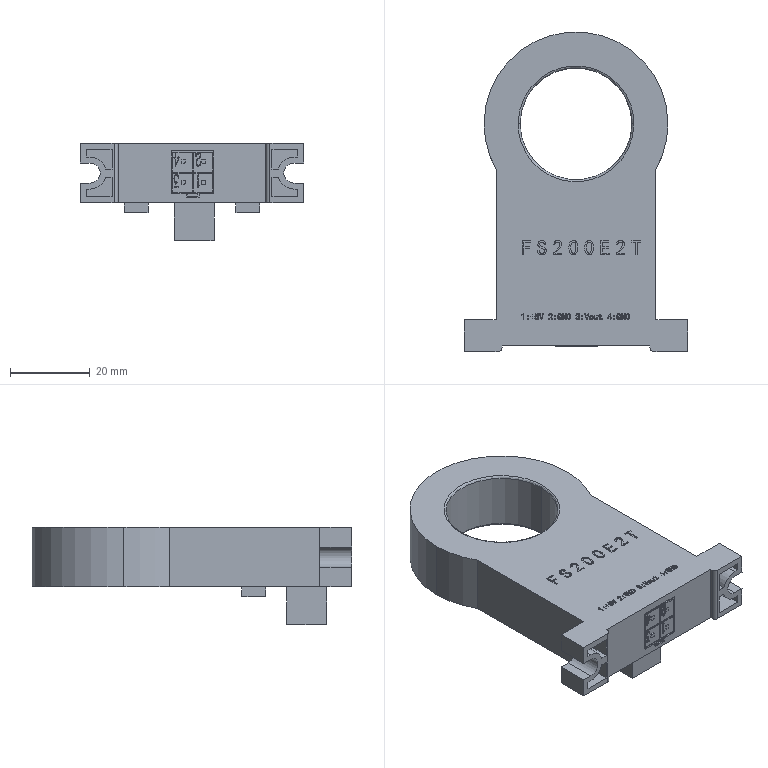Part | SolidWorks | features BaseBody 5 | 5 solids | 651 faces | box 56 x 80 x 24.3 mm | volume 37324 mm3 | plane 492 | spline 127 | cylinder 32 | commonest cylinder face diameters 0.4 x16 8 x4 4 x3 46 x3 2 x2 5 x2